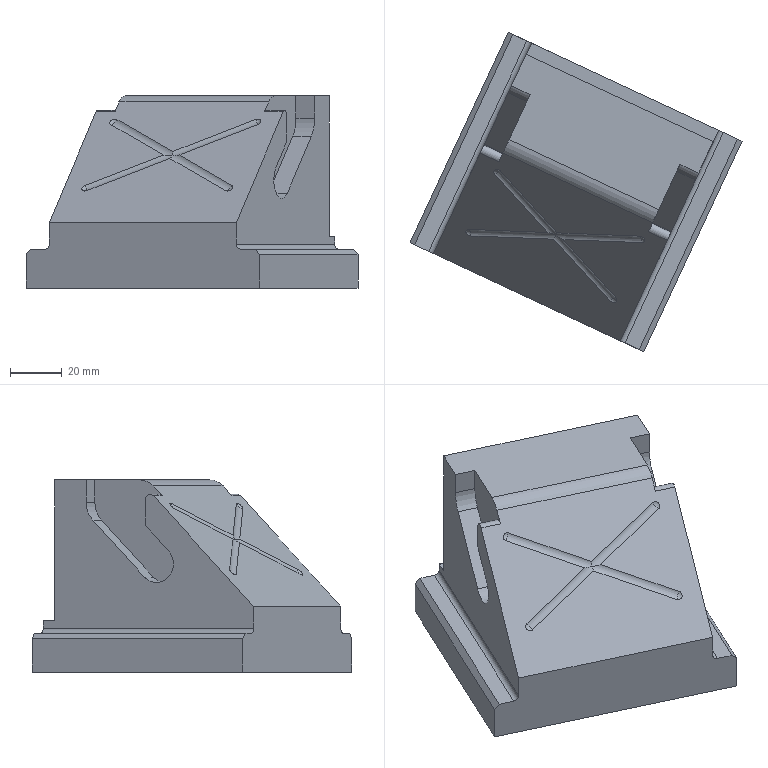Part | STEP file | gslz 2016.10.28-13_id82_x_t | 1 solid | 65 faces | box 128.666 x 123.83 x 74.5 mm | volume 424438 mm3 | plane 30 | cylinder 25 | cone 6 | sphere 4 | commonest cylinder face diameters 6 x8 4 x6 6.8 x3 8 x2 14.5 x2 20 x2